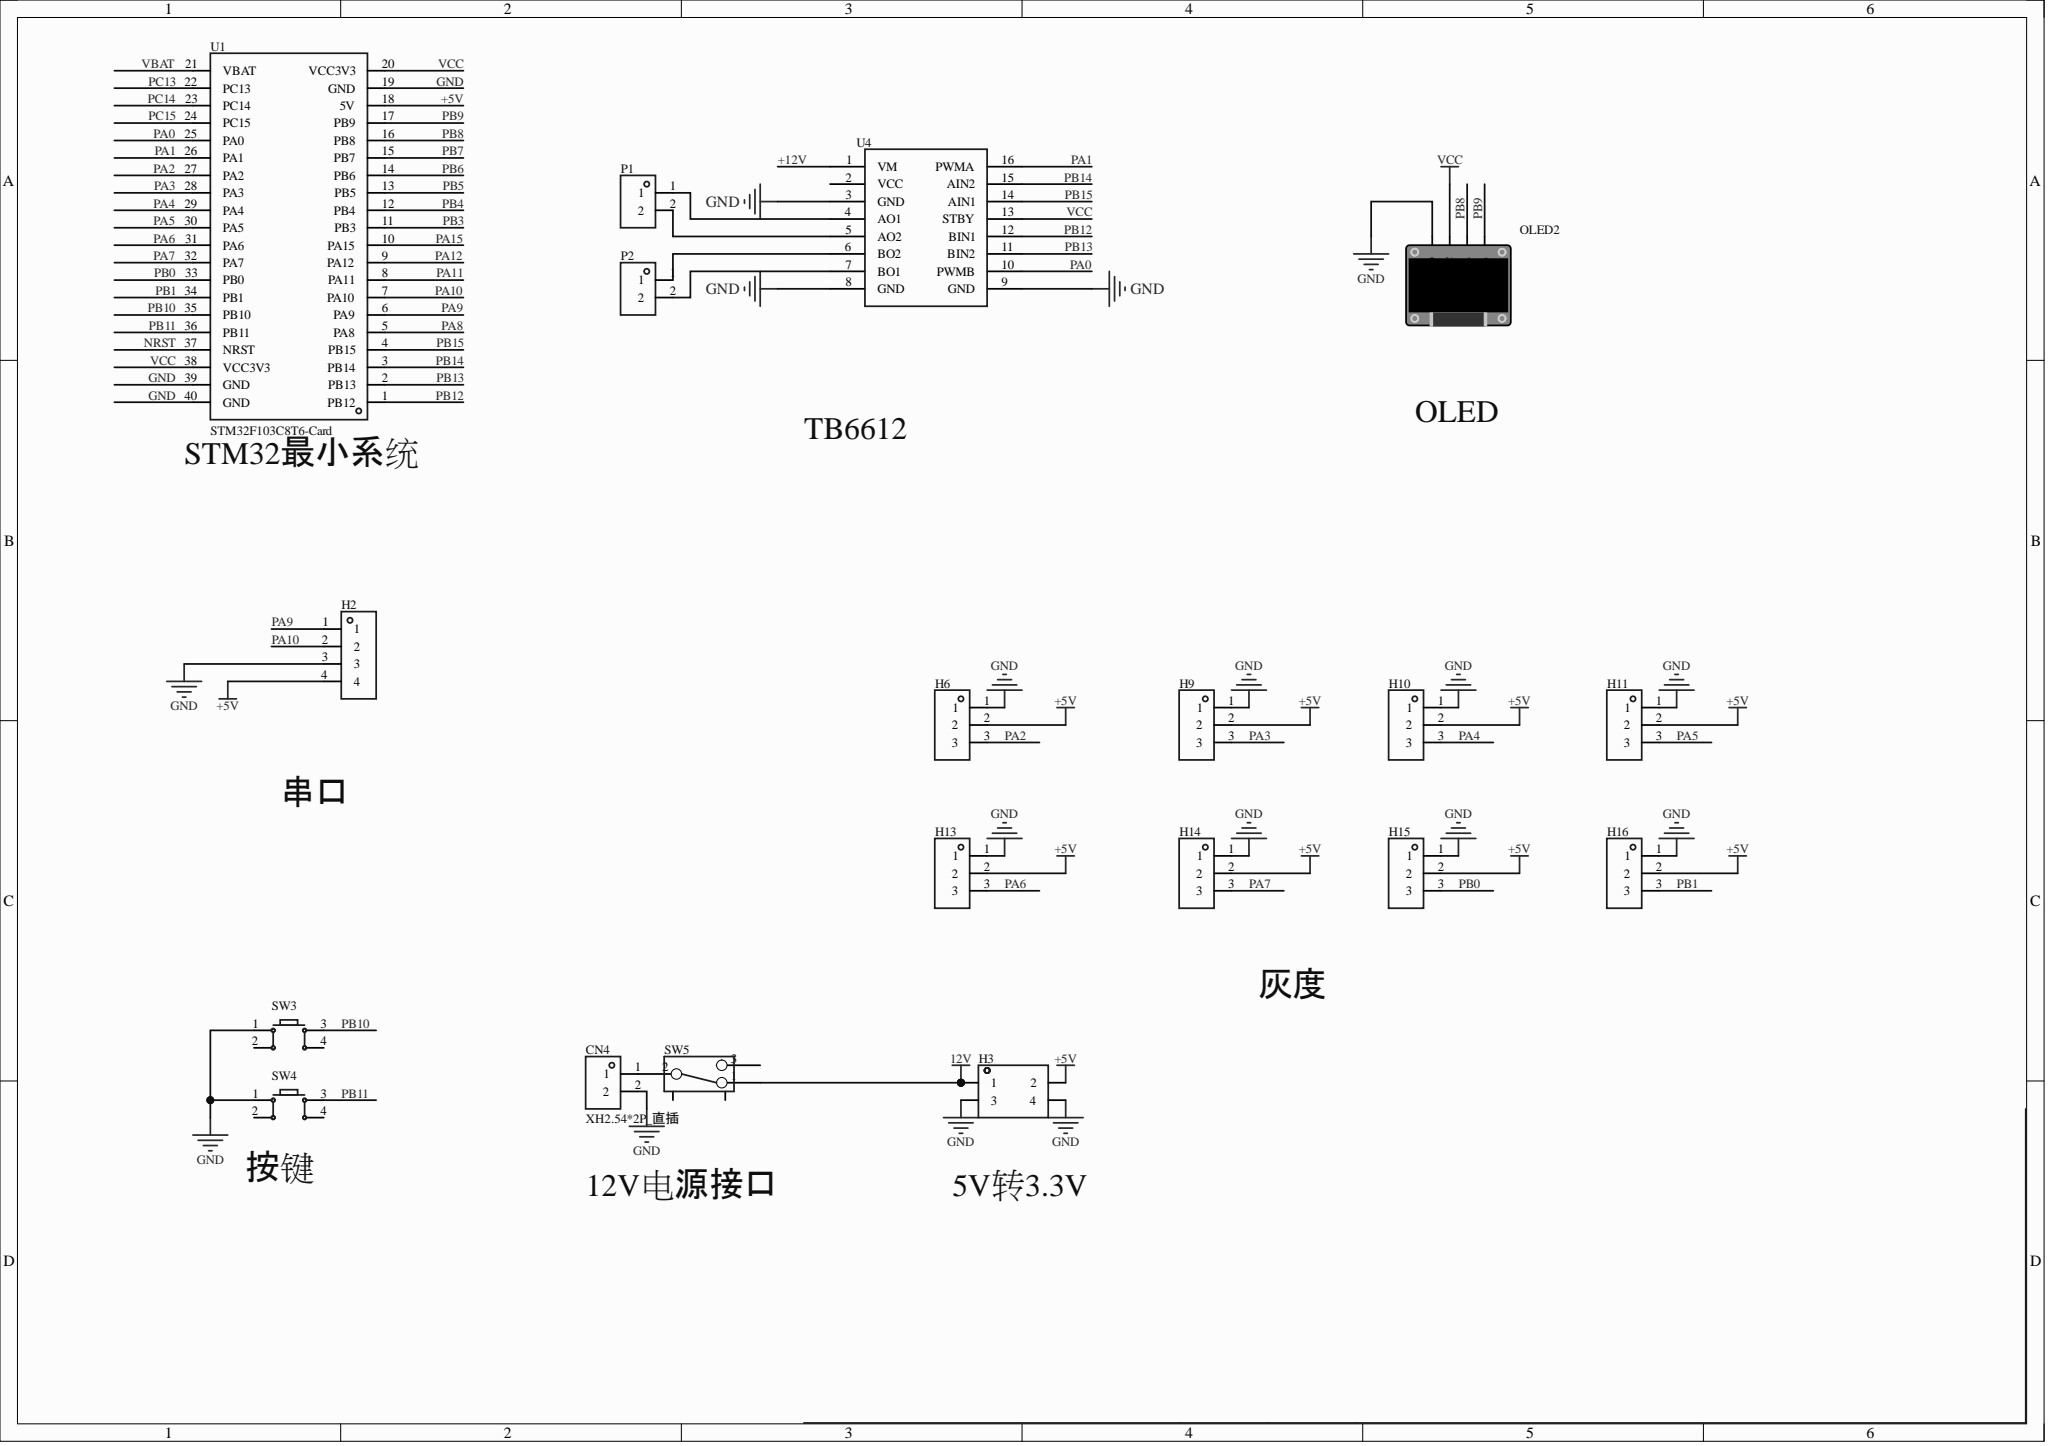Circuit board | Altium Designer | 19 parts | 29 nets
Bill of materials:
Comment,Description,Designator,Footprint,LibRef,Quantity
"XH2.54*2P_直插","","CN4","CONN-TH_2P-P2.50-XH2.54-2P","XH2.54*2P_直插","1"
"","","H2","HDR-TH_4P-P2.54-V-M","HDR-M_2.54_1x4P","1"
"","","H3","HDR-TH_4P-P2.54-V-F-R2-C2-S2.54","HDR-F_2.54_2x2","1"
"","","H6, H9, H10, H11, H13, H14, H15, H16","HDR-TH_3P-P2.54-V-F","HDR-F_2.54_1x3P","8"
"","","OLED2","0.96OLED_4P","0.96OLED模块_4P","1"
"KF301-2P接线端子","","P1, P2","CONN-TH_XY301V-A-5.0-2P","KF301-2P接线端子","2"
"","","SW3, SW4","SW-TH_4P-L6.0-W6.0-P4.50-LS6.5","Key_TH_6x6x6","2"
"","","SW5","拨动开关","拨动开关_正","1"
"STM32F103C8T6-Card","","U1","CONN-TH_L53.3-W22.9_STM32F103C8T6-CARD","STM32F103C8T6-Card","1"
"","","U4","tb6612","tb6612","1"
Netlist (Protel format):
[
CN4
CONN-TH_2P-P2.50-XH2.54-2P
XH2.54*2P_直插



]
[
H2
HDR-TH_4P-P2.54-V-M




]
[
H3
HDR-TH_4P-P2.54-V-F-R2-C2-S2.54




]
[
H6
HDR-TH_3P-P2.54-V-F




]
[
H9
HDR-TH_3P-P2.54-V-F




]
[
H10
HDR-TH_3P-P2.54-V-F




]
[
H11
HDR-TH_3P-P2.54-V-F




]
[
H13
HDR-TH_3P-P2.54-V-F




]
[
H14
HDR-TH_3P-P2.54-V-F




]
[
H15
HDR-TH_3P-P2.54-V-F




]
[
H16
HDR-TH_3P-P2.54-V-F




]
[
OLED2
0.96OLED_4P




]
[
P1
CONN-TH_XY301V-A-5.0-2P
KF301-2P接线端子



]
[
P2
CONN-TH_XY301V-A-5.0-2P
KF301-2P接线端子



]
[
SW3
SW-TH_4P-L6.0-W6.0-P4.50-LS6.5




]
[
SW4
SW-TH_4P-L6.0-W6.0-P4.50-LS6.5




]
[
SW5
拨动开关




]
[
U1
CONN-TH_L53.3-W22.9_STM32F103C8T6-CARD
STM32F103C8T6-Card



]
[
U4
tb6612




]
(
VCC
OLED2-2
U1-20
U1-38
U4-13
)
(
PB15
U1-4
U4-14
)
(
PB14
U1-3
U4-15
)
(
PB13
U1-2
U4-11
)
(
PB12
U1-1
U4-12
)
(
PB11
SW4-3
U1-36
)
(
PB10
SW3-3
U1-35
)
(
PB9
OLED2-4
U1-17
)
(
PB8
OLED2-3
U1-16
)
(
PB1
H16-3
U1-34
)
(
PB0
H15-3
U1-33
)
(
PA10
H2-2
U1-7
)
(
PA9
H2-1
U1-6
)
(
PA7
H14-3
U1-32
)
(
PA6
H13-3
U1-31
)
(
PA5
H11-3
U1-30
)
(
PA4
H10-3
U1-29
)
(
PA3
H9-3
U1-28
)
(
PA2
H6-3
U1-27
)
(
PA1
U1-26
U4-16
)
(
PA0
U1-25
U4-10
)
(
NetP2_2
P2-2
U4-7
)
(
NetP2_1
P2-1
U4-6
)
(
NetP1_2
P1-2
U4-5
)
(
NetP1_1
P1-1
U4-4
)
(
NetCN4_1
CN4-1
SW5-2
)
(
GND
CN4-2
H2-3
H3-3
H3-4
H6-1
H9-1
H10-1
H11-1
H13-1
H14-1
H15-1
H16-1
OLED2-1
SW3-1
SW4-1
U1-19
U1-39
U1-40
U4-3
U4-8
U4-9
)
(
+5V
H2-4
H3-2
H6-2
H9-2
H10-2
H11-2
H13-2
H14-2
H15-2
H16-2
U1-18
)
(
12V
H3-1
SW5-1
)